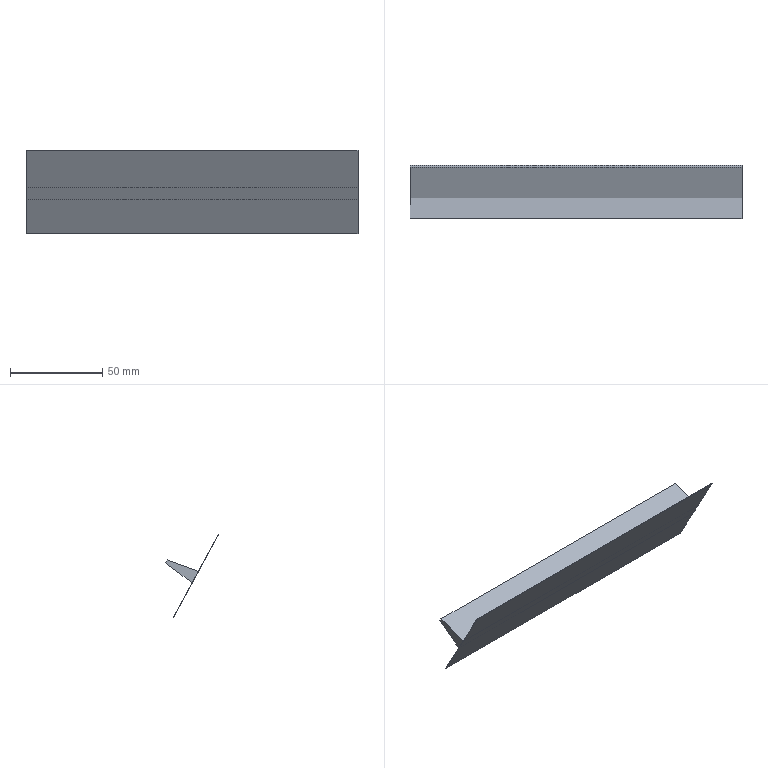Part | NX | 2 solids | 12 faces | box 180 x 28.797 x 45.12 mm | volume 16262 mm3 | plane 12
STEP:
#1=CARTESIAN_POINT('',(220.674,-533.801,2024.556));
#2=VERTEX_POINT('',#1);
#3=CARTESIAN_POINT('',(220.674,-533.961,2024.469));
#4=VERTEX_POINT('',#3);
#5=CARTESIAN_POINT('',(220.674,-533.801,2024.556));
#6=DIRECTION('',(0.,-0.8793,-0.4763));
#7=VECTOR('',#6,1.);
#8=LINE('',#5,#7);
#9=EDGE_CURVE('',#2,#4,#8,.T.);
#10=ORIENTED_EDGE('',*,*,#9,.F.);
#11=CARTESIAN_POINT('',(40.674,-533.801,2024.556));
#12=VERTEX_POINT('',#11);
#13=CARTESIAN_POINT('',(40.674,-533.801,2024.556));
#14=DIRECTION('',(1.,0.,0.));
#15=VECTOR('',#14,1.);
#16=LINE('',#13,#15);
#17=EDGE_CURVE('',#12,#2,#16,.T.);
#18=ORIENTED_EDGE('',*,*,#17,.F.);
#19=CARTESIAN_POINT('',(40.674,-533.961,2024.469));
#20=VERTEX_POINT('',#19);
#21=CARTESIAN_POINT('',(40.674,-533.801,2024.556));
#22=DIRECTION('',(0.,-0.8793,-0.4763));
#23=VECTOR('',#22,1.);
#24=LINE('',#21,#23);
#25=EDGE_CURVE('',#12,#20,#24,.T.);
#26=ORIENTED_EDGE('',*,*,#25,.T.);
#27=CARTESIAN_POINT('',(40.674,-533.961,2024.469));
#28=DIRECTION('',(1.,0.,0.));
#29=VECTOR('',#28,1.);
#30=LINE('',#27,#29);
#31=EDGE_CURVE('',#20,#4,#30,.T.);
#32=ORIENTED_EDGE('',*,*,#31,.T.);
#33=EDGE_LOOP('',(#10,#18,#26,#32));
#34=FACE_OUTER_BOUND('',#33,.T.);
#35=CARTESIAN_POINT('',(40.674,-533.801,2024.556));
#36=DIRECTION('',(0.,-0.4763,0.8793));
#37=DIRECTION('',(0.,-0.8793,-0.4763));
#38=AXIS2_PLACEMENT_3D('',#35,#36,#37);
#39=PLANE('',#38);
#40=ADVANCED_FACE('',(#34),#39,.T.);
#41=CARTESIAN_POINT('',(220.674,-509.564,1979.436));
#42=VERTEX_POINT('',#41);
#43=CARTESIAN_POINT('',(220.674,-533.961,2024.469));
#44=DIRECTION('',(0.,0.4763,-0.8793));
#45=VECTOR('',#44,1.);
#46=LINE('',#43,#45);
#47=EDGE_CURVE('',#4,#42,#46,.T.);
#48=ORIENTED_EDGE('',*,*,#47,.F.);
#49=ORIENTED_EDGE('',*,*,#31,.F.);
#50=CARTESIAN_POINT('',(40.674,-509.564,1979.436));
#51=VERTEX_POINT('',#50);
#52=CARTESIAN_POINT('',(40.674,-533.961,2024.469));
#53=DIRECTION('',(0.,0.4763,-0.8793));
#54=VECTOR('',#53,1.);
#55=LINE('',#52,#54);
#56=EDGE_CURVE('',#20,#51,#55,.T.);
#57=ORIENTED_EDGE('',*,*,#56,.T.);
#58=CARTESIAN_POINT('',(40.674,-509.564,1979.436));
#59=DIRECTION('',(1.,0.,0.));
#60=VECTOR('',#59,1.);
#61=LINE('',#58,#60);
#62=EDGE_CURVE('',#51,#42,#61,.T.);
#63=ORIENTED_EDGE('',*,*,#62,.T.);
#64=EDGE_LOOP('',(#48,#49,#57,#63));
#65=FACE_OUTER_BOUND('',#64,.T.);
#66=CARTESIAN_POINT('',(40.674,-533.961,2024.469));
#67=DIRECTION('',(0.,-0.8793,-0.4763));
#68=DIRECTION('',(0.,0.4763,-0.8793));
#69=AXIS2_PLACEMENT_3D('',#66,#67,#68);
#70=PLANE('',#69);
#71=ADVANCED_FACE('',(#65),#70,.T.);
#72=CARTESIAN_POINT('',(220.674,-509.404,1979.523));
#73=VERTEX_POINT('',#72);
#74=CARTESIAN_POINT('',(220.674,-509.564,1979.436));
#75=DIRECTION('',(0.,0.8793,0.4763));
#76=VECTOR('',#75,1.);
#77=LINE('',#74,#76);
#78=EDGE_CURVE('',#42,#73,#77,.T.);
#79=ORIENTED_EDGE('',*,*,#78,.F.);
#80=ORIENTED_EDGE('',*,*,#62,.F.);
#81=CARTESIAN_POINT('',(40.674,-509.404,1979.523));
#82=VERTEX_POINT('',#81);
#83=CARTESIAN_POINT('',(40.674,-509.564,1979.436));
#84=DIRECTION('',(0.,0.8793,0.4763));
#85=VECTOR('',#84,1.);
#86=LINE('',#83,#85);
#87=EDGE_CURVE('',#51,#82,#86,.T.);
#88=ORIENTED_EDGE('',*,*,#87,.T.);
#89=CARTESIAN_POINT('',(40.674,-509.404,1979.523));
#90=DIRECTION('',(1.,0.,0.));
#91=VECTOR('',#90,1.);
#92=LINE('',#89,#91);
#93=EDGE_CURVE('',#82,#73,#92,.T.);
#94=ORIENTED_EDGE('',*,*,#93,.T.);
#95=EDGE_LOOP('',(#79,#80,#88,#94));
#96=FACE_OUTER_BOUND('',#95,.T.);
#97=CARTESIAN_POINT('',(40.674,-509.564,1979.436));
#98=DIRECTION('',(0.,0.4763,-0.8793));
#99=DIRECTION('',(0.,0.8793,0.4763));
#100=AXIS2_PLACEMENT_3D('',#97,#98,#99);
#101=PLANE('',#100);
#102=ADVANCED_FACE('',(#96),#101,.T.);
#103=CARTESIAN_POINT('',(220.674,-509.404,1979.523));
#104=DIRECTION('',(0.,-0.4763,0.8793));
#105=VECTOR('',#104,1.);
#106=LINE('',#103,#105);
#107=EDGE_CURVE('',#73,#2,#106,.T.);
#108=ORIENTED_EDGE('',*,*,#107,.F.);
#109=ORIENTED_EDGE('',*,*,#93,.F.);
#110=CARTESIAN_POINT('',(40.674,-509.404,1979.523));
#111=DIRECTION('',(0.,-0.4763,0.8793));
#112=VECTOR('',#111,1.);
#113=LINE('',#110,#112);
#114=EDGE_CURVE('',#82,#12,#113,.T.);
#115=ORIENTED_EDGE('',*,*,#114,.T.);
#116=ORIENTED_EDGE('',*,*,#17,.T.);
#117=EDGE_LOOP('',(#108,#109,#115,#116));
#118=FACE_OUTER_BOUND('',#117,.T.);
#119=CARTESIAN_POINT('',(40.674,-509.404,1979.523));
#120=DIRECTION('',(0.,0.8793,0.4763));
#121=DIRECTION('',(0.,-0.4763,0.8793));
#122=AXIS2_PLACEMENT_3D('',#119,#120,#121);
#123=PLANE('',#122);
#124=ADVANCED_FACE('',(#118),#123,.T.);
#125=ORIENTED_EDGE('',*,*,#25,.F.);
#126=ORIENTED_EDGE('',*,*,#114,.F.);
#127=ORIENTED_EDGE('',*,*,#87,.F.);
#128=ORIENTED_EDGE('',*,*,#56,.F.);
#129=EDGE_LOOP('',(#125,#126,#127,#128));
#130=FACE_OUTER_BOUND('',#129,.T.);
#131=CARTESIAN_POINT('',(40.674,0.,0.));
#132=DIRECTION('',(1.,0.,0.));
#133=DIRECTION('',(0.,0.,-1.));
#134=AXIS2_PLACEMENT_3D('',#131,#132,#133);
#135=PLANE('',#134);
#136=ADVANCED_FACE('',(#130),#135,.F.);
#137=ORIENTED_EDGE('',*,*,#9,.T.);
#138=ORIENTED_EDGE('',*,*,#47,.T.);
#139=ORIENTED_EDGE('',*,*,#78,.T.);
#140=ORIENTED_EDGE('',*,*,#107,.T.);
#141=EDGE_LOOP('',(#137,#138,#139,#140));
#142=FACE_OUTER_BOUND('',#141,.T.);
#143=CARTESIAN_POINT('',(220.674,0.,0.));
#144=DIRECTION('',(1.,0.,0.));
#145=DIRECTION('',(0.,0.,-1.));
#146=AXIS2_PLACEMENT_3D('',#143,#144,#145);
#147=PLANE('',#146);
#148=ADVANCED_FACE('',(#142),#147,.T.);
#149=CLOSED_SHELL('',(#40,#71,#102,#124,#136,#148));
#150=MANIFOLD_SOLID_BREP('',#149);
#151=CARTESIAN_POINT('',(40.674,-523.134,2004.484));
#152=VERTEX_POINT('',#151);
#153=CARTESIAN_POINT('',(40.674,-519.704,1998.153));
#154=VERTEX_POINT('',#153);
#155=CARTESIAN_POINT('',(40.674,-519.704,1998.153));
#156=DIRECTION('',(0.,0.4763,-0.8793));
#157=VECTOR('',#156,1.);
#158=LINE('',#155,#157);
#159=EDGE_CURVE('',#152,#154,#158,.T.);
#160=ORIENTED_EDGE('',*,*,#159,.T.);
#161=CARTESIAN_POINT('',(220.674,-519.704,1998.153));
#162=VERTEX_POINT('',#161);
#163=CARTESIAN_POINT('',(220.674,-519.704,1998.153));
#164=DIRECTION('',(-1.,0.,0.));
#165=VECTOR('',#164,1.);
#166=LINE('',#163,#165);
#167=EDGE_CURVE('',#162,#154,#166,.T.);
#168=ORIENTED_EDGE('',*,*,#167,.F.);
#169=CARTESIAN_POINT('',(220.674,-523.134,2004.484));
#170=VERTEX_POINT('',#169);
#171=CARTESIAN_POINT('',(220.674,-519.704,1998.153));
#172=DIRECTION('',(0.,0.4763,-0.8793));
#173=VECTOR('',#172,1.);
#174=LINE('',#171,#173);
#175=EDGE_CURVE('',#170,#162,#174,.T.);
#176=ORIENTED_EDGE('',*,*,#175,.F.);
#177=CARTESIAN_POINT('',(220.674,-523.134,2004.484));
#178=DIRECTION('',(-1.,0.,0.));
#179=VECTOR('',#178,1.);
#180=LINE('',#177,#179);
#181=EDGE_CURVE('',#170,#152,#180,.T.);
#182=ORIENTED_EDGE('',*,*,#181,.T.);
#183=EDGE_LOOP('',(#160,#168,#176,#182));
#184=FACE_OUTER_BOUND('',#183,.T.);
#185=CARTESIAN_POINT('',(220.674,-519.704,1998.153));
#186=DIRECTION('',(0.,0.8793,0.4763));
#187=DIRECTION('',(0.,-0.4763,0.8793));
#188=AXIS2_PLACEMENT_3D('',#185,#186,#187);
#189=PLANE('',#188);
#190=ADVANCED_FACE('',(#184),#189,.F.);
#191=CARTESIAN_POINT('',(40.674,-505.164,2009.101));
#192=VERTEX_POINT('',#191);
#193=CARTESIAN_POINT('',(40.674,-505.164,2009.101));
#194=DIRECTION('',(0.,0.7989,0.6015));
#195=VECTOR('',#194,1.);
#196=LINE('',#193,#195);
#197=EDGE_CURVE('',#154,#192,#196,.T.);
#198=ORIENTED_EDGE('',*,*,#197,.T.);
#199=CARTESIAN_POINT('',(220.674,-505.164,2009.101));
#200=VERTEX_POINT('',#199);
#201=CARTESIAN_POINT('',(220.674,-505.164,2009.101));
#202=DIRECTION('',(-1.,0.,0.));
#203=VECTOR('',#202,1.);
#204=LINE('',#201,#203);
#205=EDGE_CURVE('',#200,#192,#204,.T.);
#206=ORIENTED_EDGE('',*,*,#205,.F.);
#207=CARTESIAN_POINT('',(220.674,-505.164,2009.101));
#208=DIRECTION('',(0.,0.7989,0.6015));
#209=VECTOR('',#208,1.);
#210=LINE('',#207,#209);
#211=EDGE_CURVE('',#162,#200,#210,.T.);
#212=ORIENTED_EDGE('',*,*,#211,.F.);
#213=ORIENTED_EDGE('',*,*,#167,.T.);
#214=EDGE_LOOP('',(#198,#206,#212,#213));
#215=FACE_OUTER_BOUND('',#214,.T.);
#216=CARTESIAN_POINT('',(220.674,-505.164,2009.101));
#217=DIRECTION('',(0.,-0.6015,0.7989));
#218=DIRECTION('',(0.,-0.7989,-0.6015));
#219=AXIS2_PLACEMENT_3D('',#216,#217,#218);
#220=PLANE('',#219);
#221=ADVANCED_FACE('',(#215),#220,.F.);
#222=CARTESIAN_POINT('',(40.674,-506.021,2010.684));
#223=VERTEX_POINT('',#222);
#224=CARTESIAN_POINT('',(40.674,-506.021,2010.684));
#225=DIRECTION('',(0.,-0.4763,0.8793));
#226=VECTOR('',#225,1.);
#227=LINE('',#224,#226);
#228=EDGE_CURVE('',#192,#223,#227,.T.);
#229=ORIENTED_EDGE('',*,*,#228,.T.);
#230=CARTESIAN_POINT('',(220.674,-506.021,2010.684));
#231=VERTEX_POINT('',#230);
#232=CARTESIAN_POINT('',(220.674,-506.021,2010.684));
#233=DIRECTION('',(-1.,0.,0.));
#234=VECTOR('',#233,1.);
#235=LINE('',#232,#234);
#236=EDGE_CURVE('',#231,#223,#235,.T.);
#237=ORIENTED_EDGE('',*,*,#236,.F.);
#238=CARTESIAN_POINT('',(220.674,-506.021,2010.684));
#239=DIRECTION('',(0.,-0.4763,0.8793));
#240=VECTOR('',#239,1.);
#241=LINE('',#238,#240);
#242=EDGE_CURVE('',#200,#231,#241,.T.);
#243=ORIENTED_EDGE('',*,*,#242,.F.);
#244=ORIENTED_EDGE('',*,*,#205,.T.);
#245=EDGE_LOOP('',(#229,#237,#243,#244));
#246=FACE_OUTER_BOUND('',#245,.T.);
#247=CARTESIAN_POINT('',(220.674,-506.021,2010.684));
#248=DIRECTION('',(0.,-0.8793,-0.4763));
#249=DIRECTION('',(0.,0.4763,-0.8793));
#250=AXIS2_PLACEMENT_3D('',#247,#248,#249);
#251=PLANE('',#250);
#252=ADVANCED_FACE('',(#246),#251,.F.);
#253=CARTESIAN_POINT('',(40.674,-523.134,2004.484));
#254=DIRECTION('',(0.,-0.9402,-0.3407));
#255=VECTOR('',#254,1.);
#256=LINE('',#253,#255);
#257=EDGE_CURVE('',#223,#152,#256,.T.);
#258=ORIENTED_EDGE('',*,*,#257,.T.);
#259=ORIENTED_EDGE('',*,*,#181,.F.);
#260=CARTESIAN_POINT('',(220.674,-523.134,2004.484));
#261=DIRECTION('',(0.,-0.9402,-0.3407));
#262=VECTOR('',#261,1.);
#263=LINE('',#260,#262);
#264=EDGE_CURVE('',#231,#170,#263,.T.);
#265=ORIENTED_EDGE('',*,*,#264,.F.);
#266=ORIENTED_EDGE('',*,*,#236,.T.);
#267=EDGE_LOOP('',(#258,#259,#265,#266));
#268=FACE_OUTER_BOUND('',#267,.T.);
#269=CARTESIAN_POINT('',(220.674,-523.134,2004.484));
#270=DIRECTION('',(0.,0.3407,-0.9402));
#271=DIRECTION('',(0.,0.9402,0.3407));
#272=AXIS2_PLACEMENT_3D('',#269,#270,#271);
#273=PLANE('',#272);
#274=ADVANCED_FACE('',(#268),#273,.F.);
#275=ORIENTED_EDGE('',*,*,#175,.T.);
#276=ORIENTED_EDGE('',*,*,#211,.T.);
#277=ORIENTED_EDGE('',*,*,#242,.T.);
#278=ORIENTED_EDGE('',*,*,#264,.T.);
#279=EDGE_LOOP('',(#275,#276,#277,#278));
#280=FACE_OUTER_BOUND('',#279,.T.);
#281=CARTESIAN_POINT('',(220.674,-519.704,1998.153));
#282=DIRECTION('',(1.,0.,0.));
#283=DIRECTION('',(0.,0.4763,-0.8793));
#284=AXIS2_PLACEMENT_3D('',#281,#282,#283);
#285=PLANE('',#284);
#286=ADVANCED_FACE('',(#280),#285,.T.);
#287=ORIENTED_EDGE('',*,*,#159,.F.);
#288=ORIENTED_EDGE('',*,*,#257,.F.);
#289=ORIENTED_EDGE('',*,*,#228,.F.);
#290=ORIENTED_EDGE('',*,*,#197,.F.);
#291=EDGE_LOOP('',(#287,#288,#289,#290));
#292=FACE_OUTER_BOUND('',#291,.T.);
#293=CARTESIAN_POINT('',(40.674,-519.704,1998.153));
#294=DIRECTION('',(1.,0.,0.));
#295=DIRECTION('',(0.,0.4763,-0.8793));
#296=AXIS2_PLACEMENT_3D('',#293,#294,#295);
#297=PLANE('',#296);
#298=ADVANCED_FACE('',(#292),#297,.F.);
#299=CLOSED_SHELL('',(#190,#221,#252,#274,#286,#298));
#300=MANIFOLD_SOLID_BREP('',#299);
#301=(LENGTH_UNIT()NAMED_UNIT(*)SI_UNIT(.MILLI.,.METRE.));
#302=UNCERTAINTY_MEASURE_WITH_UNIT(LENGTH_MEASURE(0.00002),#301,'','');
#303=(NAMED_UNIT(*)PLANE_ANGLE_UNIT()SI_UNIT($,.RADIAN.));
#304=PLANE_ANGLE_MEASURE_WITH_UNIT(PLANE_ANGLE_MEASURE(0.01745),#303);
#305=DIMENSIONAL_EXPONENTS(0.,0.,0.,0.,0.,0.,0.);
#306=(CONVERSION_BASED_UNIT('DEGREE',#304)NAMED_UNIT(#305)PLANE_ANGLE_UNIT());
#307=(NAMED_UNIT(*)SI_UNIT($,.STERADIAN.)SOLID_ANGLE_UNIT());
#308=(GEOMETRIC_REPRESENTATION_CONTEXT(3)GLOBAL_UNCERTAINTY_ASSIGNED_CONTEXT((#302))GLOBAL_UNIT_ASSIGNED_CONTEXT((#301,#306,#307))REPRESENTATION_CONTEXT('',''));
#309=ADVANCED_BREP_SHAPE_REPRESENTATION('',(#150,#300),#308);